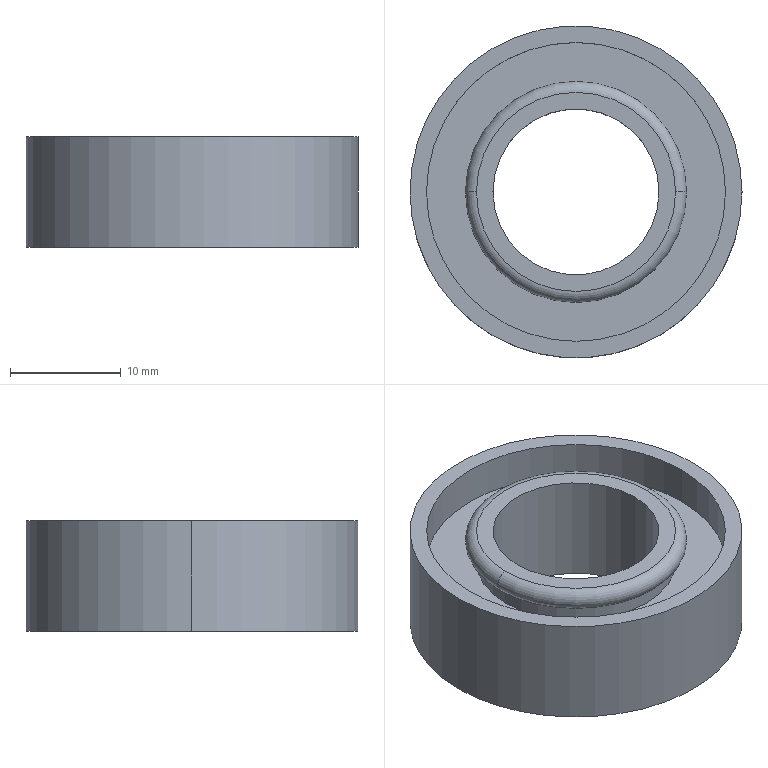Part | SolidWorks | features MirrorPattern 1, Revolution 1 | 1 solid | 22 faces | box 30 x 30 x 10 mm | volume 3261 mm3 | cylinder 12 | plane 6 | torus 4 | commonest cylinder face diameters 18 x4 27 x4 15 x2 30 x2
STEP:
#1=CARTESIAN_POINT('',(-9.,0.,5.));
#2=VERTEX_POINT('',#1);
#3=CARTESIAN_POINT('',(9.,0.,5.));
#4=VERTEX_POINT('',#3);
#5=CARTESIAN_POINT('',(0.,0.,5.));
#6=DIRECTION('',(0.,0.,1.));
#7=DIRECTION('',(1.,0.,0.));
#8=AXIS2_PLACEMENT_3D('',#5,#6,#7);
#9=CIRCLE('',#8,9.);
#10=EDGE_CURVE('',#2,#4,#9,.T.);
#11=ORIENTED_EDGE('',*,*,#10,.F.);
#12=CARTESIAN_POINT('',(-9.,0.,3.));
#13=VERTEX_POINT('',#12);
#14=CARTESIAN_POINT('',(-9.,0.,4.));
#15=DIRECTION('',(0.,-1.,0.));
#16=DIRECTION('',(1.,0.,0.));
#17=AXIS2_PLACEMENT_3D('',#14,#15,#16);
#18=CIRCLE('',#17,1.);
#19=EDGE_CURVE('',#2,#13,#18,.T.);
#20=ORIENTED_EDGE('',*,*,#19,.T.);
#21=CARTESIAN_POINT('',(9.,0.,3.));
#22=VERTEX_POINT('',#21);
#23=CARTESIAN_POINT('',(0.,0.,3.));
#24=DIRECTION('',(0.,0.,1.));
#25=DIRECTION('',(1.,0.,0.));
#26=AXIS2_PLACEMENT_3D('',#23,#24,#25);
#27=CIRCLE('',#26,9.);
#28=EDGE_CURVE('',#13,#22,#27,.T.);
#29=ORIENTED_EDGE('',*,*,#28,.T.);
#30=CARTESIAN_POINT('',(9.,0.,4.));
#31=DIRECTION('',(0.,1.,0.));
#32=DIRECTION('',(0.,0.,1.));
#33=AXIS2_PLACEMENT_3D('',#30,#31,#32);
#34=CIRCLE('',#33,1.);
#35=EDGE_CURVE('',#4,#22,#34,.T.);
#36=ORIENTED_EDGE('',*,*,#35,.F.);
#37=EDGE_LOOP('',(#11,#20,#29,#36));
#38=FACE_OUTER_BOUND('',#37,.T.);
#39=CARTESIAN_POINT('',(0.,0.,4.));
#40=DIRECTION('',(0.,0.,-1.));
#41=DIRECTION('',(1.,0.,0.));
#42=AXIS2_PLACEMENT_3D('',#39,#40,#41);
#43=TOROIDAL_SURFACE('',#42,9.,1.);
#44=ADVANCED_FACE('',(#38),#43,.T.);
#45=ORIENTED_EDGE('',*,*,#28,.F.);
#46=CARTESIAN_POINT('',(-9.,0.,1.5));
#47=VERTEX_POINT('',#46);
#48=CARTESIAN_POINT('',(-9.,0.,-4.217));
#49=DIRECTION('',(0.,0.,-1.));
#50=VECTOR('',#49,1000.);
#51=LINE('',#48,#50);
#52=EDGE_CURVE('',#13,#47,#51,.T.);
#53=ORIENTED_EDGE('',*,*,#52,.T.);
#54=CARTESIAN_POINT('',(9.,0.,1.5));
#55=VERTEX_POINT('',#54);
#56=CARTESIAN_POINT('',(0.,0.,1.5));
#57=DIRECTION('',(0.,0.,1.));
#58=DIRECTION('',(1.,0.,0.));
#59=AXIS2_PLACEMENT_3D('',#56,#57,#58);
#60=CIRCLE('',#59,9.);
#61=EDGE_CURVE('',#47,#55,#60,.T.);
#62=ORIENTED_EDGE('',*,*,#61,.T.);
#63=CARTESIAN_POINT('',(9.,0.,-4.217));
#64=DIRECTION('',(0.,0.,-1.));
#65=VECTOR('',#64,1000.);
#66=LINE('',#63,#65);
#67=EDGE_CURVE('',#22,#55,#66,.T.);
#68=ORIENTED_EDGE('',*,*,#67,.F.);
#69=EDGE_LOOP('',(#45,#53,#62,#68));
#70=FACE_OUTER_BOUND('',#69,.T.);
#71=CARTESIAN_POINT('',(0.,0.,-4.217));
#72=DIRECTION('',(0.,0.,-1.));
#73=DIRECTION('',(1.,0.,0.));
#74=AXIS2_PLACEMENT_3D('',#71,#72,#73);
#75=CYLINDRICAL_SURFACE('',#74,9.);
#76=ADVANCED_FACE('',(#70),#75,.T.);
#77=CARTESIAN_POINT('',(13.5,0.,5.));
#78=VERTEX_POINT('',#77);
#79=CARTESIAN_POINT('',(-13.5,0.,5.));
#80=VERTEX_POINT('',#79);
#81=CARTESIAN_POINT('',(0.,0.,5.));
#82=DIRECTION('',(0.,0.,1.));
#83=DIRECTION('',(1.,0.,0.));
#84=AXIS2_PLACEMENT_3D('',#81,#82,#83);
#85=CIRCLE('',#84,13.5);
#86=EDGE_CURVE('',#78,#80,#85,.T.);
#87=ORIENTED_EDGE('',*,*,#86,.T.);
#88=CARTESIAN_POINT('',(-13.5,0.,1.5));
#89=VERTEX_POINT('',#88);
#90=CARTESIAN_POINT('',(-13.5,0.,-4.217));
#91=DIRECTION('',(0.,0.,-1.));
#92=VECTOR('',#91,1000.);
#93=LINE('',#90,#92);
#94=EDGE_CURVE('',#80,#89,#93,.T.);
#95=ORIENTED_EDGE('',*,*,#94,.T.);
#96=CARTESIAN_POINT('',(13.5,0.,1.5));
#97=VERTEX_POINT('',#96);
#98=CARTESIAN_POINT('',(0.,0.,1.5));
#99=DIRECTION('',(0.,0.,1.));
#100=DIRECTION('',(1.,0.,0.));
#101=AXIS2_PLACEMENT_3D('',#98,#99,#100);
#102=CIRCLE('',#101,13.5);
#103=EDGE_CURVE('',#97,#89,#102,.T.);
#104=ORIENTED_EDGE('',*,*,#103,.F.);
#105=CARTESIAN_POINT('',(13.5,0.,-4.217));
#106=DIRECTION('',(0.,0.,-1.));
#107=VECTOR('',#106,1000.);
#108=LINE('',#105,#107);
#109=EDGE_CURVE('',#78,#97,#108,.T.);
#110=ORIENTED_EDGE('',*,*,#109,.F.);
#111=EDGE_LOOP('',(#87,#95,#104,#110));
#112=FACE_OUTER_BOUND('',#111,.T.);
#113=CARTESIAN_POINT('',(0.,0.,-4.217));
#114=DIRECTION('',(0.,0.,-1.));
#115=DIRECTION('',(1.,0.,0.));
#116=AXIS2_PLACEMENT_3D('',#113,#114,#115);
#117=CYLINDRICAL_SURFACE('',#116,13.5);
#118=ADVANCED_FACE('',(#112),#117,.F.);
#119=CARTESIAN_POINT('',(-7.5,0.,-5.));
#120=VERTEX_POINT('',#119);
#121=CARTESIAN_POINT('',(7.5,0.,-5.));
#122=VERTEX_POINT('',#121);
#123=CARTESIAN_POINT('',(0.,0.,-5.));
#124=DIRECTION('',(0.,0.,1.));
#125=DIRECTION('',(1.,0.,0.));
#126=AXIS2_PLACEMENT_3D('',#123,#124,#125);
#127=CIRCLE('',#126,7.5);
#128=EDGE_CURVE('',#120,#122,#127,.T.);
#129=ORIENTED_EDGE('',*,*,#128,.F.);
#130=CARTESIAN_POINT('',(-7.5,0.,5.));
#131=VERTEX_POINT('',#130);
#132=CARTESIAN_POINT('',(-7.5,0.,4.217));
#133=DIRECTION('',(0.,0.,1.));
#134=VECTOR('',#133,1000.);
#135=LINE('',#132,#134);
#136=EDGE_CURVE('',#120,#131,#135,.T.);
#137=ORIENTED_EDGE('',*,*,#136,.T.);
#138=CARTESIAN_POINT('',(7.5,0.,5.));
#139=VERTEX_POINT('',#138);
#140=CARTESIAN_POINT('',(0.,0.,5.));
#141=DIRECTION('',(0.,0.,1.));
#142=DIRECTION('',(1.,0.,0.));
#143=AXIS2_PLACEMENT_3D('',#140,#141,#142);
#144=CIRCLE('',#143,7.5);
#145=EDGE_CURVE('',#131,#139,#144,.T.);
#146=ORIENTED_EDGE('',*,*,#145,.T.);
#147=CARTESIAN_POINT('',(7.5,0.,4.217));
#148=DIRECTION('',(0.,0.,1.));
#149=VECTOR('',#148,1000.);
#150=LINE('',#147,#149);
#151=EDGE_CURVE('',#122,#139,#150,.T.);
#152=ORIENTED_EDGE('',*,*,#151,.F.);
#153=EDGE_LOOP('',(#129,#137,#146,#152));
#154=FACE_OUTER_BOUND('',#153,.T.);
#155=CARTESIAN_POINT('',(0.,0.,4.217));
#156=DIRECTION('',(0.,0.,1.));
#157=DIRECTION('',(1.,0.,0.));
#158=AXIS2_PLACEMENT_3D('',#155,#156,#157);
#159=CYLINDRICAL_SURFACE('',#158,7.5);
#160=ADVANCED_FACE('',(#154),#159,.F.);
#161=CARTESIAN_POINT('',(9.,0.,-5.));
#162=VERTEX_POINT('',#161);
#163=CARTESIAN_POINT('',(-9.,0.,-5.));
#164=VERTEX_POINT('',#163);
#165=CARTESIAN_POINT('',(0.,0.,-5.));
#166=DIRECTION('',(0.,0.,1.));
#167=DIRECTION('',(1.,0.,0.));
#168=AXIS2_PLACEMENT_3D('',#165,#166,#167);
#169=CIRCLE('',#168,9.);
#170=EDGE_CURVE('',#162,#164,#169,.T.);
#171=ORIENTED_EDGE('',*,*,#170,.T.);
#172=CARTESIAN_POINT('',(-9.,0.,-3.));
#173=VERTEX_POINT('',#172);
#174=CARTESIAN_POINT('',(-9.,0.,-4.));
#175=DIRECTION('',(0.,1.,0.));
#176=DIRECTION('',(-1.,0.,0.));
#177=AXIS2_PLACEMENT_3D('',#174,#175,#176);
#178=CIRCLE('',#177,1.);
#179=EDGE_CURVE('',#164,#173,#178,.T.);
#180=ORIENTED_EDGE('',*,*,#179,.T.);
#181=CARTESIAN_POINT('',(9.,0.,-3.));
#182=VERTEX_POINT('',#181);
#183=CARTESIAN_POINT('',(0.,0.,-3.));
#184=DIRECTION('',(0.,0.,1.));
#185=DIRECTION('',(1.,0.,0.));
#186=AXIS2_PLACEMENT_3D('',#183,#184,#185);
#187=CIRCLE('',#186,9.);
#188=EDGE_CURVE('',#182,#173,#187,.T.);
#189=ORIENTED_EDGE('',*,*,#188,.F.);
#190=CARTESIAN_POINT('',(9.,0.,-4.));
#191=DIRECTION('',(0.,-1.,0.));
#192=DIRECTION('',(0.,0.,-1.));
#193=AXIS2_PLACEMENT_3D('',#190,#191,#192);
#194=CIRCLE('',#193,1.);
#195=EDGE_CURVE('',#162,#182,#194,.T.);
#196=ORIENTED_EDGE('',*,*,#195,.F.);
#197=EDGE_LOOP('',(#171,#180,#189,#196));
#198=FACE_OUTER_BOUND('',#197,.T.);
#199=CARTESIAN_POINT('',(0.,0.,-4.));
#200=DIRECTION('',(0.,0.,1.));
#201=DIRECTION('',(1.,0.,0.));
#202=AXIS2_PLACEMENT_3D('',#199,#200,#201);
#203=TOROIDAL_SURFACE('',#202,9.,1.);
#204=ADVANCED_FACE('',(#198),#203,.T.);
#205=ORIENTED_EDGE('',*,*,#188,.T.);
#206=CARTESIAN_POINT('',(-9.,0.,-1.5));
#207=VERTEX_POINT('',#206);
#208=CARTESIAN_POINT('',(-9.,0.,4.217));
#209=DIRECTION('',(0.,0.,1.));
#210=VECTOR('',#209,1000.);
#211=LINE('',#208,#210);
#212=EDGE_CURVE('',#173,#207,#211,.T.);
#213=ORIENTED_EDGE('',*,*,#212,.T.);
#214=CARTESIAN_POINT('',(9.,0.,-1.5));
#215=VERTEX_POINT('',#214);
#216=CARTESIAN_POINT('',(0.,0.,-1.5));
#217=DIRECTION('',(0.,0.,1.));
#218=DIRECTION('',(1.,0.,0.));
#219=AXIS2_PLACEMENT_3D('',#216,#217,#218);
#220=CIRCLE('',#219,9.);
#221=EDGE_CURVE('',#215,#207,#220,.T.);
#222=ORIENTED_EDGE('',*,*,#221,.F.);
#223=CARTESIAN_POINT('',(9.,0.,4.217));
#224=DIRECTION('',(0.,0.,1.));
#225=VECTOR('',#224,1000.);
#226=LINE('',#223,#225);
#227=EDGE_CURVE('',#182,#215,#226,.T.);
#228=ORIENTED_EDGE('',*,*,#227,.F.);
#229=EDGE_LOOP('',(#205,#213,#222,#228));
#230=FACE_OUTER_BOUND('',#229,.T.);
#231=CARTESIAN_POINT('',(0.,0.,4.217));
#232=DIRECTION('',(0.,0.,1.));
#233=DIRECTION('',(1.,0.,0.));
#234=AXIS2_PLACEMENT_3D('',#231,#232,#233);
#235=CYLINDRICAL_SURFACE('',#234,9.);
#236=ADVANCED_FACE('',(#230),#235,.T.);
#237=CARTESIAN_POINT('',(-13.5,0.,-5.));
#238=VERTEX_POINT('',#237);
#239=CARTESIAN_POINT('',(13.5,0.,-5.));
#240=VERTEX_POINT('',#239);
#241=CARTESIAN_POINT('',(0.,0.,-5.));
#242=DIRECTION('',(0.,0.,1.));
#243=DIRECTION('',(1.,0.,0.));
#244=AXIS2_PLACEMENT_3D('',#241,#242,#243);
#245=CIRCLE('',#244,13.5);
#246=EDGE_CURVE('',#238,#240,#245,.T.);
#247=ORIENTED_EDGE('',*,*,#246,.F.);
#248=CARTESIAN_POINT('',(-13.5,0.,-1.5));
#249=VERTEX_POINT('',#248);
#250=CARTESIAN_POINT('',(-13.5,0.,4.217));
#251=DIRECTION('',(0.,0.,1.));
#252=VECTOR('',#251,1000.);
#253=LINE('',#250,#252);
#254=EDGE_CURVE('',#238,#249,#253,.T.);
#255=ORIENTED_EDGE('',*,*,#254,.T.);
#256=CARTESIAN_POINT('',(13.5,0.,-1.5));
#257=VERTEX_POINT('',#256);
#258=CARTESIAN_POINT('',(0.,0.,-1.5));
#259=DIRECTION('',(0.,0.,1.));
#260=DIRECTION('',(1.,0.,0.));
#261=AXIS2_PLACEMENT_3D('',#258,#259,#260);
#262=CIRCLE('',#261,13.5);
#263=EDGE_CURVE('',#249,#257,#262,.T.);
#264=ORIENTED_EDGE('',*,*,#263,.T.);
#265=CARTESIAN_POINT('',(13.5,0.,4.217));
#266=DIRECTION('',(0.,0.,1.));
#267=VECTOR('',#266,1000.);
#268=LINE('',#265,#267);
#269=EDGE_CURVE('',#240,#257,#268,.T.);
#270=ORIENTED_EDGE('',*,*,#269,.F.);
#271=EDGE_LOOP('',(#247,#255,#264,#270));
#272=FACE_OUTER_BOUND('',#271,.T.);
#273=CARTESIAN_POINT('',(0.,0.,4.217));
#274=DIRECTION('',(0.,0.,1.));
#275=DIRECTION('',(1.,0.,0.));
#276=AXIS2_PLACEMENT_3D('',#273,#274,#275);
#277=CYLINDRICAL_SURFACE('',#276,13.5);
#278=ADVANCED_FACE('',(#272),#277,.F.);
#279=CARTESIAN_POINT('',(15.,0.,-5.));
#280=VERTEX_POINT('',#279);
#281=CARTESIAN_POINT('',(-15.,0.,-5.));
#282=VERTEX_POINT('',#281);
#283=CARTESIAN_POINT('',(0.,0.,-5.));
#284=DIRECTION('',(0.,0.,1.));
#285=DIRECTION('',(1.,0.,0.));
#286=AXIS2_PLACEMENT_3D('',#283,#284,#285);
#287=CIRCLE('',#286,15.);
#288=EDGE_CURVE('',#280,#282,#287,.T.);
#289=ORIENTED_EDGE('',*,*,#288,.T.);
#290=CARTESIAN_POINT('',(-15.,0.,5.));
#291=VERTEX_POINT('',#290);
#292=CARTESIAN_POINT('',(-15.,0.,4.217));
#293=DIRECTION('',(0.,0.,1.));
#294=VECTOR('',#293,1000.);
#295=LINE('',#292,#294);
#296=EDGE_CURVE('',#282,#291,#295,.T.);
#297=ORIENTED_EDGE('',*,*,#296,.T.);
#298=CARTESIAN_POINT('',(15.,0.,5.));
#299=VERTEX_POINT('',#298);
#300=CARTESIAN_POINT('',(0.,0.,5.));
#301=DIRECTION('',(0.,0.,1.));
#302=DIRECTION('',(1.,0.,0.));
#303=AXIS2_PLACEMENT_3D('',#300,#301,#302);
#304=CIRCLE('',#303,15.);
#305=EDGE_CURVE('',#299,#291,#304,.T.);
#306=ORIENTED_EDGE('',*,*,#305,.F.);
#307=CARTESIAN_POINT('',(15.,0.,4.217));
#308=DIRECTION('',(0.,0.,1.));
#309=VECTOR('',#308,1000.);
#310=LINE('',#307,#309);
#311=EDGE_CURVE('',#280,#299,#310,.T.);
#312=ORIENTED_EDGE('',*,*,#311,.F.);
#313=EDGE_LOOP('',(#289,#297,#306,#312));
#314=FACE_OUTER_BOUND('',#313,.T.);
#315=CARTESIAN_POINT('',(0.,0.,4.217));
#316=DIRECTION('',(0.,0.,1.));
#317=DIRECTION('',(1.,0.,0.));
#318=AXIS2_PLACEMENT_3D('',#315,#316,#317);
#319=CYLINDRICAL_SURFACE('',#318,15.);
#320=ADVANCED_FACE('',(#314),#319,.T.);
#321=ORIENTED_EDGE('',*,*,#296,.F.);
#322=CARTESIAN_POINT('',(0.,0.,-5.));
#323=DIRECTION('',(0.,0.,1.));
#324=DIRECTION('',(1.,0.,0.));
#325=AXIS2_PLACEMENT_3D('',#322,#323,#324);
#326=CIRCLE('',#325,15.);
#327=EDGE_CURVE('',#282,#280,#326,.T.);
#328=ORIENTED_EDGE('',*,*,#327,.T.);
#329=ORIENTED_EDGE('',*,*,#311,.T.);
#330=CARTESIAN_POINT('',(0.,0.,5.));
#331=DIRECTION('',(0.,0.,1.));
#332=DIRECTION('',(1.,0.,0.));
#333=AXIS2_PLACEMENT_3D('',#330,#331,#332);
#334=CIRCLE('',#333,15.);
#335=EDGE_CURVE('',#291,#299,#334,.T.);
#336=ORIENTED_EDGE('',*,*,#335,.F.);
#337=EDGE_LOOP('',(#321,#328,#329,#336));
#338=FACE_OUTER_BOUND('',#337,.T.);
#339=CARTESIAN_POINT('',(0.,0.,4.217));
#340=DIRECTION('',(0.,0.,1.));
#341=DIRECTION('',(1.,0.,0.));
#342=AXIS2_PLACEMENT_3D('',#339,#340,#341);
#343=CYLINDRICAL_SURFACE('',#342,15.);
#344=ADVANCED_FACE('',(#338),#343,.T.);
#345=ORIENTED_EDGE('',*,*,#288,.F.);
#346=ORIENTED_EDGE('',*,*,#327,.F.);
#347=EDGE_LOOP('',(#345,#346));
#348=FACE_OUTER_BOUND('',#347,.T.);
#349=CARTESIAN_POINT('',(0.,0.,-5.));
#350=DIRECTION('',(0.,0.,1.));
#351=DIRECTION('',(1.,0.,0.));
#352=AXIS2_PLACEMENT_3D('',#349,#350,#351);
#353=CIRCLE('',#352,13.5);
#354=EDGE_CURVE('',#240,#238,#353,.T.);
#355=ORIENTED_EDGE('',*,*,#354,.T.);
#356=ORIENTED_EDGE('',*,*,#246,.T.);
#357=EDGE_LOOP('',(#355,#356));
#358=FACE_BOUND('',#357,.T.);
#359=CARTESIAN_POINT('',(0.,15.,-5.));
#360=DIRECTION('',(0.,0.,1.));
#361=DIRECTION('',(1.,0.,0.));
#362=AXIS2_PLACEMENT_3D('',#359,#360,#361);
#363=PLANE('',#362);
#364=ADVANCED_FACE('',(#348,#358),#363,.F.);
#365=ORIENTED_EDGE('',*,*,#254,.F.);
#366=ORIENTED_EDGE('',*,*,#354,.F.);
#367=ORIENTED_EDGE('',*,*,#269,.T.);
#368=CARTESIAN_POINT('',(0.,0.,-1.5));
#369=DIRECTION('',(0.,0.,1.));
#370=DIRECTION('',(1.,0.,0.));
#371=AXIS2_PLACEMENT_3D('',#368,#369,#370);
#372=CIRCLE('',#371,13.5);
#373=EDGE_CURVE('',#257,#249,#372,.T.);
#374=ORIENTED_EDGE('',*,*,#373,.T.);
#375=EDGE_LOOP('',(#365,#366,#367,#374));
#376=FACE_OUTER_BOUND('',#375,.T.);
#377=CARTESIAN_POINT('',(0.,0.,4.217));
#378=DIRECTION('',(0.,0.,1.));
#379=DIRECTION('',(1.,0.,0.));
#380=AXIS2_PLACEMENT_3D('',#377,#378,#379);
#381=CYLINDRICAL_SURFACE('',#380,13.5);
#382=ADVANCED_FACE('',(#376),#381,.F.);
#383=ORIENTED_EDGE('',*,*,#373,.F.);
#384=ORIENTED_EDGE('',*,*,#263,.F.);
#385=EDGE_LOOP('',(#383,#384));
#386=FACE_OUTER_BOUND('',#385,.T.);
#387=ORIENTED_EDGE('',*,*,#221,.T.);
#388=CARTESIAN_POINT('',(0.,0.,-1.5));
#389=DIRECTION('',(0.,0.,1.));
#390=DIRECTION('',(1.,0.,0.));
#391=AXIS2_PLACEMENT_3D('',#388,#389,#390);
#392=CIRCLE('',#391,9.);
#393=EDGE_CURVE('',#207,#215,#392,.T.);
#394=ORIENTED_EDGE('',*,*,#393,.T.);
#395=EDGE_LOOP('',(#387,#394));
#396=FACE_BOUND('',#395,.T.);
#397=CARTESIAN_POINT('',(0.,9.,-1.5));
#398=DIRECTION('',(0.,0.,1.));
#399=DIRECTION('',(1.,0.,0.));
#400=AXIS2_PLACEMENT_3D('',#397,#398,#399);
#401=PLANE('',#400);
#402=ADVANCED_FACE('',(#386,#396),#401,.F.);
#403=ORIENTED_EDGE('',*,*,#212,.F.);
#404=CARTESIAN_POINT('',(0.,0.,-3.));
#405=DIRECTION('',(0.,0.,1.));
#406=DIRECTION('',(1.,0.,0.));
#407=AXIS2_PLACEMENT_3D('',#404,#405,#406);
#408=CIRCLE('',#407,9.);
#409=EDGE_CURVE('',#173,#182,#408,.T.);
#410=ORIENTED_EDGE('',*,*,#409,.T.);
#411=ORIENTED_EDGE('',*,*,#227,.T.);
#412=ORIENTED_EDGE('',*,*,#393,.F.);
#413=EDGE_LOOP('',(#403,#410,#411,#412));
#414=FACE_OUTER_BOUND('',#413,.T.);
#415=CARTESIAN_POINT('',(0.,0.,4.217));
#416=DIRECTION('',(0.,0.,1.));
#417=DIRECTION('',(1.,0.,0.));
#418=AXIS2_PLACEMENT_3D('',#415,#416,#417);
#419=CYLINDRICAL_SURFACE('',#418,9.);
#420=ADVANCED_FACE('',(#414),#419,.T.);
#421=ORIENTED_EDGE('',*,*,#179,.F.);
#422=CARTESIAN_POINT('',(0.,0.,-5.));
#423=DIRECTION('',(0.,0.,1.));
#424=DIRECTION('',(1.,0.,0.));
#425=AXIS2_PLACEMENT_3D('',#422,#423,#424);
#426=CIRCLE('',#425,9.);
#427=EDGE_CURVE('',#164,#162,#426,.T.);
#428=ORIENTED_EDGE('',*,*,#427,.T.);
#429=ORIENTED_EDGE('',*,*,#195,.T.);
#430=ORIENTED_EDGE('',*,*,#409,.F.);
#431=EDGE_LOOP('',(#421,#428,#429,#430));
#432=FACE_OUTER_BOUND('',#431,.T.);
#433=CARTESIAN_POINT('',(0.,0.,-4.));
#434=DIRECTION('',(0.,0.,1.));
#435=DIRECTION('',(1.,0.,0.));
#436=AXIS2_PLACEMENT_3D('',#433,#434,#435);
#437=TOROIDAL_SURFACE('',#436,9.,1.);
#438=ADVANCED_FACE('',(#432),#437,.T.);
#439=ORIENTED_EDGE('',*,*,#170,.F.);
#440=ORIENTED_EDGE('',*,*,#427,.F.);
#441=EDGE_LOOP('',(#439,#440));
#442=FACE_OUTER_BOUND('',#441,.T.);
#443=CARTESIAN_POINT('',(0.,0.,-5.));
#444=DIRECTION('',(0.,0.,1.));
#445=DIRECTION('',(1.,0.,0.));
#446=AXIS2_PLACEMENT_3D('',#443,#444,#445);
#447=CIRCLE('',#446,7.5);
#448=EDGE_CURVE('',#122,#120,#447,.T.);
#449=ORIENTED_EDGE('',*,*,#448,.T.);
#450=ORIENTED_EDGE('',*,*,#128,.T.);
#451=EDGE_LOOP('',(#449,#450));
#452=FACE_BOUND('',#451,.T.);
#453=CARTESIAN_POINT('',(0.,7.5,-5.));
#454=DIRECTION('',(0.,0.,1.));
#455=DIRECTION('',(1.,0.,0.));
#456=AXIS2_PLACEMENT_3D('',#453,#454,#455);
#457=PLANE('',#456);
#458=ADVANCED_FACE('',(#442,#452),#457,.F.);
#459=ORIENTED_EDGE('',*,*,#136,.F.);
#460=ORIENTED_EDGE('',*,*,#448,.F.);
#461=ORIENTED_EDGE('',*,*,#151,.T.);
#462=CARTESIAN_POINT('',(0.,0.,5.));
#463=DIRECTION('',(0.,0.,1.));
#464=DIRECTION('',(1.,0.,0.));
#465=AXIS2_PLACEMENT_3D('',#462,#463,#464);
#466=CIRCLE('',#465,7.5);
#467=EDGE_CURVE('',#139,#131,#466,.T.);
#468=ORIENTED_EDGE('',*,*,#467,.T.);
#469=EDGE_LOOP('',(#459,#460,#461,#468));
#470=FACE_OUTER_BOUND('',#469,.T.);
#471=CARTESIAN_POINT('',(0.,0.,4.217));
#472=DIRECTION('',(0.,0.,1.));
#473=DIRECTION('',(1.,0.,0.));
#474=AXIS2_PLACEMENT_3D('',#471,#472,#473);
#475=CYLINDRICAL_SURFACE('',#474,7.5);
#476=ADVANCED_FACE('',(#470),#475,.F.);
#477=ORIENTED_EDGE('',*,*,#305,.T.);
#478=ORIENTED_EDGE('',*,*,#335,.T.);
#479=EDGE_LOOP('',(#477,#478));
#480=FACE_OUTER_BOUND('',#479,.T.);
#481=ORIENTED_EDGE('',*,*,#86,.F.);
#482=CARTESIAN_POINT('',(0.,0.,5.));
#483=DIRECTION('',(0.,0.,1.));
#484=DIRECTION('',(1.,0.,0.));
#485=AXIS2_PLACEMENT_3D('',#482,#483,#484);
#486=CIRCLE('',#485,13.5);
#487=EDGE_CURVE('',#80,#78,#486,.T.);
#488=ORIENTED_EDGE('',*,*,#487,.F.);
#489=EDGE_LOOP('',(#481,#488));
#490=FACE_BOUND('',#489,.T.);
#491=CARTESIAN_POINT('',(0.,15.,5.));
#492=DIRECTION('',(0.,0.,-1.));
#493=DIRECTION('',(1.,0.,0.));
#494=AXIS2_PLACEMENT_3D('',#491,#492,#493);
#495=PLANE('',#494);
#496=ADVANCED_FACE('',(#480,#490),#495,.F.);
#497=ORIENTED_EDGE('',*,*,#94,.F.);
#498=ORIENTED_EDGE('',*,*,#487,.T.);
#499=ORIENTED_EDGE('',*,*,#109,.T.);
#500=CARTESIAN_POINT('',(0.,0.,1.5));
#501=DIRECTION('',(0.,0.,1.));
#502=DIRECTION('',(1.,0.,0.));
#503=AXIS2_PLACEMENT_3D('',#500,#501,#502);
#504=CIRCLE('',#503,13.5);
#505=EDGE_CURVE('',#89,#97,#504,.T.);
#506=ORIENTED_EDGE('',*,*,#505,.F.);
#507=EDGE_LOOP('',(#497,#498,#499,#506));
#508=FACE_OUTER_BOUND('',#507,.T.);
#509=CARTESIAN_POINT('',(0.,0.,-4.217));
#510=DIRECTION('',(0.,0.,-1.));
#511=DIRECTION('',(1.,0.,0.));
#512=AXIS2_PLACEMENT_3D('',#509,#510,#511);
#513=CYLINDRICAL_SURFACE('',#512,13.5);
#514=ADVANCED_FACE('',(#508),#513,.F.);
#515=ORIENTED_EDGE('',*,*,#103,.T.);
#516=ORIENTED_EDGE('',*,*,#505,.T.);
#517=EDGE_LOOP('',(#515,#516));
#518=FACE_OUTER_BOUND('',#517,.T.);
#519=CARTESIAN_POINT('',(0.,0.,1.5));
#520=DIRECTION('',(0.,0.,1.));
#521=DIRECTION('',(1.,0.,0.));
#522=AXIS2_PLACEMENT_3D('',#519,#520,#521);
#523=CIRCLE('',#522,9.);
#524=EDGE_CURVE('',#55,#47,#523,.T.);
#525=ORIENTED_EDGE('',*,*,#524,.F.);
#526=ORIENTED_EDGE('',*,*,#61,.F.);
#527=EDGE_LOOP('',(#525,#526));
#528=FACE_BOUND('',#527,.T.);
#529=CARTESIAN_POINT('',(0.,9.,1.5));
#530=DIRECTION('',(0.,0.,-1.));
#531=DIRECTION('',(1.,0.,0.));
#532=AXIS2_PLACEMENT_3D('',#529,#530,#531);
#533=PLANE('',#532);
#534=ADVANCED_FACE('',(#518,#528),#533,.F.);
#535=ORIENTED_EDGE('',*,*,#52,.F.);
#536=CARTESIAN_POINT('',(0.,0.,3.));
#537=DIRECTION('',(0.,0.,1.));
#538=DIRECTION('',(1.,0.,0.));
#539=AXIS2_PLACEMENT_3D('',#536,#537,#538);
#540=CIRCLE('',#539,9.);
#541=EDGE_CURVE('',#22,#13,#540,.T.);
#542=ORIENTED_EDGE('',*,*,#541,.F.);
#543=ORIENTED_EDGE('',*,*,#67,.T.);
#544=ORIENTED_EDGE('',*,*,#524,.T.);
#545=EDGE_LOOP('',(#535,#542,#543,#544));
#546=FACE_OUTER_BOUND('',#545,.T.);
#547=CARTESIAN_POINT('',(0.,0.,-4.217));
#548=DIRECTION('',(0.,0.,-1.));
#549=DIRECTION('',(1.,0.,0.));
#550=AXIS2_PLACEMENT_3D('',#547,#548,#549);
#551=CYLINDRICAL_SURFACE('',#550,9.);
#552=ADVANCED_FACE('',(#546),#551,.T.);
#553=ORIENTED_EDGE('',*,*,#19,.F.);
#554=CARTESIAN_POINT('',(0.,0.,5.));
#555=DIRECTION('',(0.,0.,1.));
#556=DIRECTION('',(1.,0.,0.));
#557=AXIS2_PLACEMENT_3D('',#554,#555,#556);
#558=CIRCLE('',#557,9.);
#559=EDGE_CURVE('',#4,#2,#558,.T.);
#560=ORIENTED_EDGE('',*,*,#559,.F.);
#561=ORIENTED_EDGE('',*,*,#35,.T.);
#562=ORIENTED_EDGE('',*,*,#541,.T.);
#563=EDGE_LOOP('',(#553,#560,#561,#562));
#564=FACE_OUTER_BOUND('',#563,.T.);
#565=CARTESIAN_POINT('',(0.,0.,4.));
#566=DIRECTION('',(0.,0.,-1.));
#567=DIRECTION('',(1.,0.,0.));
#568=AXIS2_PLACEMENT_3D('',#565,#566,#567);
#569=TOROIDAL_SURFACE('',#568,9.,1.);
#570=ADVANCED_FACE('',(#564),#569,.T.);
#571=ORIENTED_EDGE('',*,*,#559,.T.);
#572=ORIENTED_EDGE('',*,*,#10,.T.);
#573=EDGE_LOOP('',(#571,#572));
#574=FACE_OUTER_BOUND('',#573,.T.);
#575=ORIENTED_EDGE('',*,*,#467,.F.);
#576=ORIENTED_EDGE('',*,*,#145,.F.);
#577=EDGE_LOOP('',(#575,#576));
#578=FACE_BOUND('',#577,.T.);
#579=CARTESIAN_POINT('',(0.,7.5,5.));
#580=DIRECTION('',(0.,0.,-1.));
#581=DIRECTION('',(1.,0.,0.));
#582=AXIS2_PLACEMENT_3D('',#579,#580,#581);
#583=PLANE('',#582);
#584=ADVANCED_FACE('',(#574,#578),#583,.F.);
#585=CLOSED_SHELL('',(#44,#76,#118,#160,#204,#236,#278,#320,#344,#364,#382,#402,#420,#438,#458,#476,#496,#514,#534,#552,#570,#584));
#586=MANIFOLD_SOLID_BREP('',#585);
#587=CARTESIAN_POINT('',(0.,0.,0.));
#588=DIRECTION('',(0.,0.,1.));
#589=DIRECTION('',(1.,0.,0.));
#590=AXIS2_PLACEMENT_3D('',#587,#588,#589);
#591=(LENGTH_UNIT()NAMED_UNIT(*)SI_UNIT(.MILLI.,.METRE.));
#592=UNCERTAINTY_MEASURE_WITH_UNIT(LENGTH_MEASURE(0.00001),#591,'','');
#593=(NAMED_UNIT(*)PLANE_ANGLE_UNIT()SI_UNIT($,.RADIAN.));
#594=(NAMED_UNIT(*)SI_UNIT($,.STERADIAN.)SOLID_ANGLE_UNIT());
#595=(GEOMETRIC_REPRESENTATION_CONTEXT(3)GLOBAL_UNCERTAINTY_ASSIGNED_CONTEXT((#592))GLOBAL_UNIT_ASSIGNED_CONTEXT((#591,#593,#594))REPRESENTATION_CONTEXT('',''));
#596=ADVANCED_BREP_SHAPE_REPRESENTATION('',(#586,#590),#595);